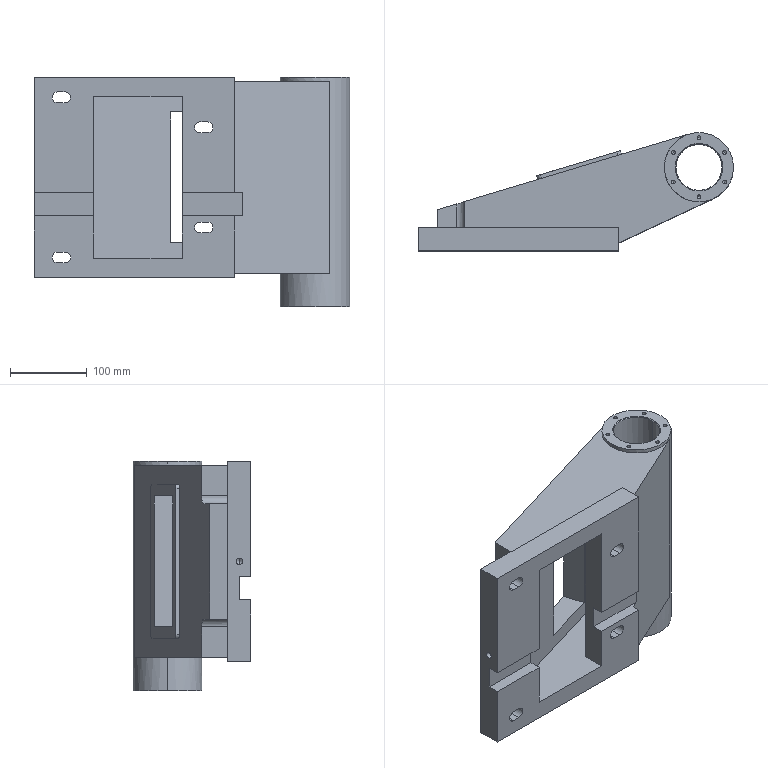Part | STEP file | 400v80 Tailstock | 1 solid | 124 faces | box 409.5 x 153.533 x 298 mm | volume 5552005 mm3 | plane 49 | cylinder 45 | cone 30 | commonest cylinder face diameters 5 x24 14 x8 10 x4 8.5 x2 20 x2 60 x2